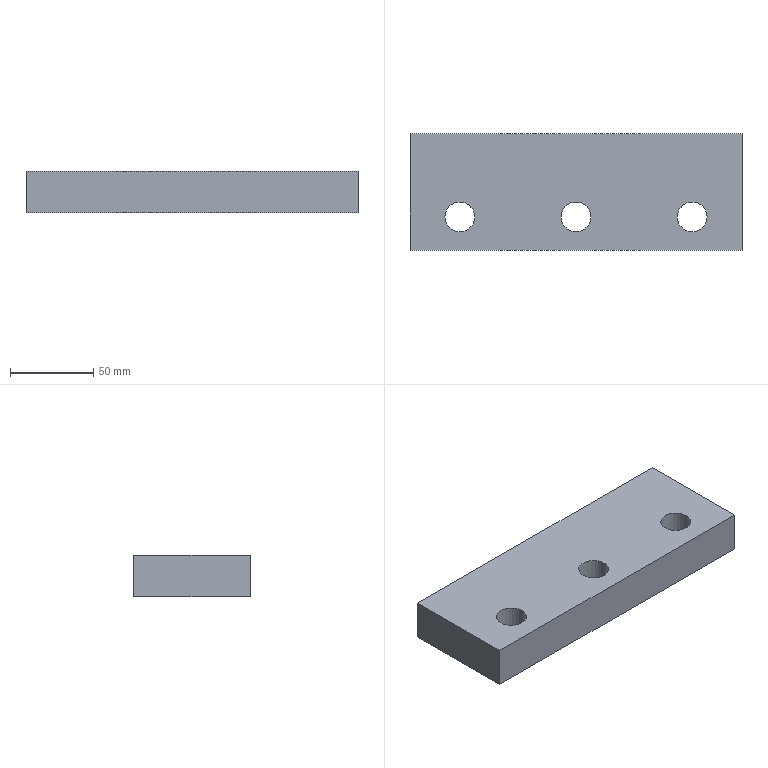Part | NX | features solid 2 | 1 solid | 9 faces | box 200 x 70 x 25 mm | volume 330915 mm3 | plane 6 | cylinder 3 | commonest cylinder face diameters 18 x3
STEP:
#1=CARTESIAN_POINT('',(857.5,-453.,92.));
#2=VERTEX_POINT('',#1);
#3=CARTESIAN_POINT('',(857.5,-453.,117.));
#4=VERTEX_POINT('',#3);
#5=CARTESIAN_POINT('',(857.5,-453.,117.));
#6=DIRECTION('',(0.,0.,-1.));
#7=VECTOR('',#6,1000.);
#8=LINE('',#5,#7);
#9=EDGE_CURVE('',#2,#4,#8,.F.);
#10=ORIENTED_EDGE('',*,*,#9,.F.);
#11=CARTESIAN_POINT('',(1057.5,-453.,92.));
#12=VERTEX_POINT('',#11);
#13=CARTESIAN_POINT('',(797.5,-453.,92.));
#14=DIRECTION('',(-1.,0.,0.));
#15=VECTOR('',#14,1000.);
#16=LINE('',#13,#15);
#17=EDGE_CURVE('',#2,#12,#16,.F.);
#18=ORIENTED_EDGE('',*,*,#17,.T.);
#19=CARTESIAN_POINT('',(1057.5,-453.,117.));
#20=VERTEX_POINT('',#19);
#21=CARTESIAN_POINT('',(1057.5,-453.,117.));
#22=DIRECTION('',(0.,0.,1.));
#23=VECTOR('',#22,1000.);
#24=LINE('',#21,#23);
#25=EDGE_CURVE('',#12,#20,#24,.T.);
#26=ORIENTED_EDGE('',*,*,#25,.T.);
#27=CARTESIAN_POINT('',(797.5,-453.,117.));
#28=DIRECTION('',(1.,0.,0.));
#29=VECTOR('',#28,1000.);
#30=LINE('',#27,#29);
#31=EDGE_CURVE('',#4,#20,#30,.T.);
#32=ORIENTED_EDGE('',*,*,#31,.F.);
#33=EDGE_LOOP('',(#10,#18,#26,#32));
#34=FACE_BOUND('',#33,.T.);
#35=CARTESIAN_POINT('',(797.5,-453.,117.));
#36=DIRECTION('',(0.,-1.,0.));
#37=DIRECTION('',(1.,0.,0.));
#38=AXIS2_PLACEMENT_3D('',#35,#36,#37);
#39=PLANE('',#38);
#40=ADVANCED_FACE('',(#34),#39,.T.);
#41=ORIENTED_EDGE('',*,*,#25,.F.);
#42=CARTESIAN_POINT('',(1057.5,-383.,92.));
#43=VERTEX_POINT('',#42);
#44=CARTESIAN_POINT('',(1057.5,-453.,92.));
#45=DIRECTION('',(0.,-1.,0.));
#46=VECTOR('',#45,1000.);
#47=LINE('',#44,#46);
#48=EDGE_CURVE('',#12,#43,#47,.F.);
#49=ORIENTED_EDGE('',*,*,#48,.T.);
#50=CARTESIAN_POINT('',(1057.5,-383.,117.));
#51=VERTEX_POINT('',#50);
#52=CARTESIAN_POINT('',(1057.5,-383.,117.));
#53=DIRECTION('',(0.,0.,-1.));
#54=VECTOR('',#53,1000.);
#55=LINE('',#52,#54);
#56=EDGE_CURVE('',#43,#51,#55,.F.);
#57=ORIENTED_EDGE('',*,*,#56,.T.);
#58=CARTESIAN_POINT('',(1057.5,-453.,117.));
#59=DIRECTION('',(0.,-1.,0.));
#60=VECTOR('',#59,1000.);
#61=LINE('',#58,#60);
#62=EDGE_CURVE('',#20,#51,#61,.F.);
#63=ORIENTED_EDGE('',*,*,#62,.F.);
#64=EDGE_LOOP('',(#41,#49,#57,#63));
#65=FACE_BOUND('',#64,.T.);
#66=CARTESIAN_POINT('',(1057.5,-453.,117.));
#67=DIRECTION('',(1.,0.,0.));
#68=DIRECTION('',(0.,1.,0.));
#69=AXIS2_PLACEMENT_3D('',#66,#67,#68);
#70=PLANE('',#69);
#71=ADVANCED_FACE('',(#65),#70,.T.);
#72=ORIENTED_EDGE('',*,*,#56,.F.);
#73=CARTESIAN_POINT('',(857.5,-383.,92.));
#74=VERTEX_POINT('',#73);
#75=CARTESIAN_POINT('',(797.5,-383.,92.));
#76=DIRECTION('',(1.,0.,0.));
#77=VECTOR('',#76,1000.);
#78=LINE('',#75,#77);
#79=EDGE_CURVE('',#74,#43,#78,.T.);
#80=ORIENTED_EDGE('',*,*,#79,.F.);
#81=CARTESIAN_POINT('',(857.5,-383.,117.));
#82=VERTEX_POINT('',#81);
#83=CARTESIAN_POINT('',(857.5,-383.,117.));
#84=DIRECTION('',(0.,0.,1.));
#85=VECTOR('',#84,1000.);
#86=LINE('',#83,#85);
#87=EDGE_CURVE('',#74,#82,#86,.T.);
#88=ORIENTED_EDGE('',*,*,#87,.T.);
#89=CARTESIAN_POINT('',(797.5,-383.,117.));
#90=DIRECTION('',(1.,0.,0.));
#91=VECTOR('',#90,1000.);
#92=LINE('',#89,#91);
#93=EDGE_CURVE('',#82,#51,#92,.T.);
#94=ORIENTED_EDGE('',*,*,#93,.T.);
#95=EDGE_LOOP('',(#72,#80,#88,#94));
#96=FACE_BOUND('',#95,.T.);
#97=CARTESIAN_POINT('',(797.5,-383.,117.));
#98=DIRECTION('',(0.,-1.,0.));
#99=DIRECTION('',(1.,0.,0.));
#100=AXIS2_PLACEMENT_3D('',#97,#98,#99);
#101=PLANE('',#100);
#102=ADVANCED_FACE('',(#96),#101,.F.);
#103=CARTESIAN_POINT('',(857.5,-453.,92.));
#104=DIRECTION('',(0.,1.,0.));
#105=VECTOR('',#104,1000.);
#106=LINE('',#103,#105);
#107=EDGE_CURVE('',#2,#74,#106,.T.);
#108=ORIENTED_EDGE('',*,*,#107,.F.);
#109=ORIENTED_EDGE('',*,*,#9,.T.);
#110=CARTESIAN_POINT('',(857.5,-453.,117.));
#111=DIRECTION('',(0.,1.,0.));
#112=VECTOR('',#111,1000.);
#113=LINE('',#110,#112);
#114=EDGE_CURVE('',#4,#82,#113,.T.);
#115=ORIENTED_EDGE('',*,*,#114,.T.);
#116=ORIENTED_EDGE('',*,*,#87,.F.);
#117=EDGE_LOOP('',(#108,#109,#115,#116));
#118=FACE_BOUND('',#117,.T.);
#119=CARTESIAN_POINT('',(857.5,-453.,117.));
#120=DIRECTION('',(1.,0.,0.));
#121=DIRECTION('',(0.,1.,0.));
#122=AXIS2_PLACEMENT_3D('',#119,#120,#121);
#123=PLANE('',#122);
#124=ADVANCED_FACE('',(#118),#123,.F.);
#125=CARTESIAN_POINT('',(966.5,-433.,117.));
#126=VERTEX_POINT('',#125);
#127=CARTESIAN_POINT('',(957.5,-433.,117.));
#128=DIRECTION('',(0.,0.,-1.));
#129=DIRECTION('',(1.,0.,0.));
#130=AXIS2_PLACEMENT_3D('',#127,#128,#129);
#131=CIRCLE('',#130,9.);
#132=EDGE_CURVE('',#126,#126,#131,.T.);
#133=ORIENTED_EDGE('',*,*,#132,.T.);
#134=EDGE_LOOP('',(#133));
#135=FACE_BOUND('',#134,.T.);
#136=CARTESIAN_POINT('',(896.5,-433.,117.));
#137=VERTEX_POINT('',#136);
#138=CARTESIAN_POINT('',(887.5,-433.,117.));
#139=DIRECTION('',(0.,0.,-1.));
#140=DIRECTION('',(1.,0.,0.));
#141=AXIS2_PLACEMENT_3D('',#138,#139,#140);
#142=CIRCLE('',#141,9.);
#143=EDGE_CURVE('',#137,#137,#142,.T.);
#144=ORIENTED_EDGE('',*,*,#143,.T.);
#145=EDGE_LOOP('',(#144));
#146=FACE_BOUND('',#145,.T.);
#147=CARTESIAN_POINT('',(1036.5,-433.,117.));
#148=VERTEX_POINT('',#147);
#149=CARTESIAN_POINT('',(1027.5,-433.,117.));
#150=DIRECTION('',(0.,0.,-1.));
#151=DIRECTION('',(1.,0.,0.));
#152=AXIS2_PLACEMENT_3D('',#149,#150,#151);
#153=CIRCLE('',#152,9.);
#154=EDGE_CURVE('',#148,#148,#153,.T.);
#155=ORIENTED_EDGE('',*,*,#154,.T.);
#156=EDGE_LOOP('',(#155));
#157=FACE_BOUND('',#156,.T.);
#158=ORIENTED_EDGE('',*,*,#93,.F.);
#159=ORIENTED_EDGE('',*,*,#114,.F.);
#160=ORIENTED_EDGE('',*,*,#31,.T.);
#161=ORIENTED_EDGE('',*,*,#62,.T.);
#162=EDGE_LOOP('',(#158,#159,#160,#161));
#163=FACE_BOUND('',#162,.T.);
#164=CARTESIAN_POINT('',(797.5,-453.,117.));
#165=DIRECTION('',(0.,0.,-1.));
#166=DIRECTION('',(1.,0.,0.));
#167=AXIS2_PLACEMENT_3D('',#164,#165,#166);
#168=PLANE('',#167);
#169=ADVANCED_FACE('',(#135,#146,#157,#163),#168,.F.);
#170=CARTESIAN_POINT('',(966.5,-433.,92.));
#171=VERTEX_POINT('',#170);
#172=CARTESIAN_POINT('',(957.5,-433.,92.));
#173=DIRECTION('',(0.,0.,-1.));
#174=DIRECTION('',(1.,0.,0.));
#175=AXIS2_PLACEMENT_3D('',#172,#173,#174);
#176=CIRCLE('',#175,9.);
#177=EDGE_CURVE('',#171,#171,#176,.F.);
#178=ORIENTED_EDGE('',*,*,#177,.T.);
#179=EDGE_LOOP('',(#178));
#180=FACE_BOUND('',#179,.T.);
#181=CARTESIAN_POINT('',(896.5,-433.,92.));
#182=VERTEX_POINT('',#181);
#183=CARTESIAN_POINT('',(887.5,-433.,92.));
#184=DIRECTION('',(0.,0.,-1.));
#185=DIRECTION('',(1.,0.,0.));
#186=AXIS2_PLACEMENT_3D('',#183,#184,#185);
#187=CIRCLE('',#186,9.);
#188=EDGE_CURVE('',#182,#182,#187,.F.);
#189=ORIENTED_EDGE('',*,*,#188,.T.);
#190=EDGE_LOOP('',(#189));
#191=FACE_BOUND('',#190,.T.);
#192=CARTESIAN_POINT('',(1036.5,-433.,92.));
#193=VERTEX_POINT('',#192);
#194=CARTESIAN_POINT('',(1027.5,-433.,92.));
#195=DIRECTION('',(0.,0.,-1.));
#196=DIRECTION('',(1.,0.,0.));
#197=AXIS2_PLACEMENT_3D('',#194,#195,#196);
#198=CIRCLE('',#197,9.);
#199=EDGE_CURVE('',#193,#193,#198,.F.);
#200=ORIENTED_EDGE('',*,*,#199,.T.);
#201=EDGE_LOOP('',(#200));
#202=FACE_BOUND('',#201,.T.);
#203=ORIENTED_EDGE('',*,*,#79,.T.);
#204=ORIENTED_EDGE('',*,*,#48,.F.);
#205=ORIENTED_EDGE('',*,*,#17,.F.);
#206=ORIENTED_EDGE('',*,*,#107,.T.);
#207=EDGE_LOOP('',(#203,#204,#205,#206));
#208=FACE_BOUND('',#207,.T.);
#209=CARTESIAN_POINT('',(797.5,-453.,92.));
#210=DIRECTION('',(0.,0.,-1.));
#211=DIRECTION('',(1.,0.,0.));
#212=AXIS2_PLACEMENT_3D('',#209,#210,#211);
#213=PLANE('',#212);
#214=ADVANCED_FACE('',(#180,#191,#202,#208),#213,.T.);
#215=ORIENTED_EDGE('',*,*,#199,.F.);
#216=EDGE_LOOP('',(#215));
#217=FACE_BOUND('',#216,.T.);
#218=ORIENTED_EDGE('',*,*,#154,.F.);
#219=EDGE_LOOP('',(#218));
#220=FACE_BOUND('',#219,.T.);
#221=CARTESIAN_POINT('',(1027.5,-433.,97.));
#222=DIRECTION('',(0.,0.,1.));
#223=DIRECTION('',(-1.,0.,0.));
#224=AXIS2_PLACEMENT_3D('',#221,#222,#223);
#225=CYLINDRICAL_SURFACE('',#224,9.);
#226=ADVANCED_FACE('',(#217,#220),#225,.F.);
#227=ORIENTED_EDGE('',*,*,#188,.F.);
#228=EDGE_LOOP('',(#227));
#229=FACE_BOUND('',#228,.T.);
#230=ORIENTED_EDGE('',*,*,#143,.F.);
#231=EDGE_LOOP('',(#230));
#232=FACE_BOUND('',#231,.T.);
#233=CARTESIAN_POINT('',(887.5,-433.,97.));
#234=DIRECTION('',(0.,0.,1.));
#235=DIRECTION('',(-1.,0.,0.));
#236=AXIS2_PLACEMENT_3D('',#233,#234,#235);
#237=CYLINDRICAL_SURFACE('',#236,9.);
#238=ADVANCED_FACE('',(#229,#232),#237,.F.);
#239=ORIENTED_EDGE('',*,*,#177,.F.);
#240=EDGE_LOOP('',(#239));
#241=FACE_BOUND('',#240,.T.);
#242=ORIENTED_EDGE('',*,*,#132,.F.);
#243=EDGE_LOOP('',(#242));
#244=FACE_BOUND('',#243,.T.);
#245=CARTESIAN_POINT('',(957.5,-433.,97.));
#246=DIRECTION('',(0.,0.,1.));
#247=DIRECTION('',(-1.,0.,0.));
#248=AXIS2_PLACEMENT_3D('',#245,#246,#247);
#249=CYLINDRICAL_SURFACE('',#248,9.);
#250=ADVANCED_FACE('',(#241,#244),#249,.F.);
#251=CLOSED_SHELL('',(#40,#71,#102,#124,#169,#214,#226,#238,#250));
#252=MANIFOLD_SOLID_BREP('',#251);
#253=(LENGTH_UNIT()NAMED_UNIT(*)SI_UNIT(.MILLI.,.METRE.));
#254=UNCERTAINTY_MEASURE_WITH_UNIT(LENGTH_MEASURE(0.00001),#253,'','');
#255=(NAMED_UNIT(*)PLANE_ANGLE_UNIT()SI_UNIT($,.RADIAN.));
#256=(NAMED_UNIT(*)SI_UNIT($,.STERADIAN.)SOLID_ANGLE_UNIT());
#257=(GEOMETRIC_REPRESENTATION_CONTEXT(3)GLOBAL_UNCERTAINTY_ASSIGNED_CONTEXT((#254))GLOBAL_UNIT_ASSIGNED_CONTEXT((#253,#255,#256))REPRESENTATION_CONTEXT('',''));
#258=ADVANCED_BREP_SHAPE_REPRESENTATION('',(#252),#257);